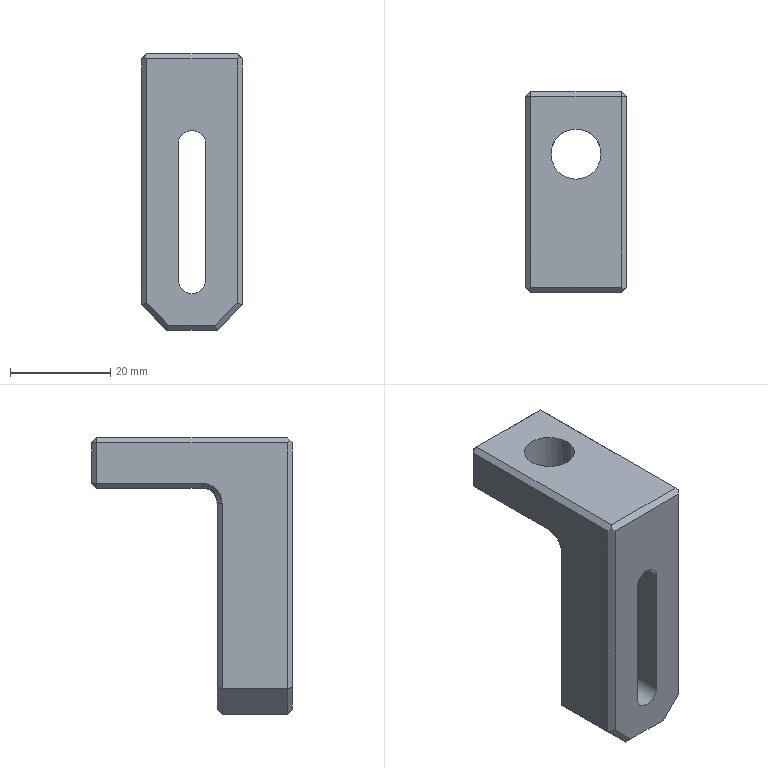Part | Creo | 1 solid | 47 faces | box 20 x 40 x 55 mm | volume 16524 mm3 | plane 38 | cylinder 7 | cone 2 | commonest cylinder face diameters 10 x4 5.5 x2 6 x1
STEP:
#1=CARTESIAN_POINT('',(-227.177,414.995,-19.5));
#2=VERTEX_POINT('',#1);
#3=CARTESIAN_POINT('',(-209.177,414.995,-19.5));
#4=VERTEX_POINT('',#3);
#5=CARTESIAN_POINT('',(-227.177,414.995,-19.5));
#6=DIRECTION('',(1.,0.,0.));
#7=VECTOR('',#6,18.);
#8=LINE('',#5,#7);
#9=EDGE_CURVE('',#2,#4,#8,.T.);
#10=ORIENTED_EDGE('',*,*,#9,.T.);
#11=CARTESIAN_POINT('',(-209.177,414.995,-11.5));
#12=VERTEX_POINT('',#11);
#13=CARTESIAN_POINT('',(-209.177,414.995,-19.5));
#14=DIRECTION('',(0.,0.,1.));
#15=VECTOR('',#14,8.);
#16=LINE('',#13,#15);
#17=EDGE_CURVE('',#4,#12,#16,.T.);
#18=ORIENTED_EDGE('',*,*,#17,.T.);
#19=CARTESIAN_POINT('',(-227.177,414.995,-11.5));
#20=VERTEX_POINT('',#19);
#21=CARTESIAN_POINT('',(-209.177,414.995,-11.5));
#22=DIRECTION('',(-1.,0.,0.));
#23=VECTOR('',#22,18.);
#24=LINE('',#21,#23);
#25=EDGE_CURVE('',#12,#20,#24,.T.);
#26=ORIENTED_EDGE('',*,*,#25,.T.);
#27=CARTESIAN_POINT('',(-227.177,414.995,-11.5));
#28=DIRECTION('',(0.,0.,-1.));
#29=VECTOR('',#28,8.);
#30=LINE('',#27,#29);
#31=EDGE_CURVE('',#20,#2,#30,.T.);
#32=ORIENTED_EDGE('',*,*,#31,.T.);
#33=EDGE_LOOP('',(#10,#18,#26,#32));
#34=FACE_OUTER_BOUND('',#33,.F.);
#35=CARTESIAN_POINT('',(-218.177,414.995,-33.));
#36=DIRECTION('',(0.,1.,0.));
#37=DIRECTION('',(0.,0.,-1.));
#38=AXIS2_PLACEMENT_3D('',#35,#36,#37);
#39=PLANE('',#38);
#40=ADVANCED_FACE('',(#34),#39,.T.);
#41=CARTESIAN_POINT('',(-209.177,413.995,-20.5));
#42=VERTEX_POINT('',#41);
#43=CARTESIAN_POINT('',(-209.177,413.995,-20.5));
#44=DIRECTION('',(0.,0.7071,0.7071));
#45=VECTOR('',#44,1.414);
#46=LINE('',#43,#45);
#47=EDGE_CURVE('',#42,#4,#46,.T.);
#48=ORIENTED_EDGE('',*,*,#47,.T.);
#49=ORIENTED_EDGE('',*,*,#9,.F.);
#50=CARTESIAN_POINT('',(-227.177,413.995,-20.5));
#51=VERTEX_POINT('',#50);
#52=CARTESIAN_POINT('',(-227.177,413.995,-20.5));
#53=DIRECTION('',(0.,0.7071,0.7071));
#54=VECTOR('',#53,1.414);
#55=LINE('',#52,#54);
#56=EDGE_CURVE('',#51,#2,#55,.T.);
#57=ORIENTED_EDGE('',*,*,#56,.F.);
#58=CARTESIAN_POINT('',(-209.177,413.995,-20.5));
#59=DIRECTION('',(-1.,0.,0.));
#60=VECTOR('',#59,18.);
#61=LINE('',#58,#60);
#62=EDGE_CURVE('',#42,#51,#61,.T.);
#63=ORIENTED_EDGE('',*,*,#62,.F.);
#64=EDGE_LOOP('',(#48,#49,#57,#63));
#65=FACE_OUTER_BOUND('',#64,.F.);
#66=CARTESIAN_POINT('',(-218.177,413.995,-20.5));
#67=DIRECTION('',(0.,0.7071,-0.7071));
#68=DIRECTION('',(1.,0.,0.));
#69=AXIS2_PLACEMENT_3D('',#66,#67,#68);
#70=PLANE('',#69);
#71=ADVANCED_FACE('',(#65),#70,.T.);
#72=CARTESIAN_POINT('',(-208.177,413.995,-19.5));
#73=VERTEX_POINT('',#72);
#74=CARTESIAN_POINT('',(-209.177,414.995,-19.5));
#75=DIRECTION('',(0.7071,-0.7071,0.));
#76=VECTOR('',#75,1.414);
#77=LINE('',#74,#76);
#78=EDGE_CURVE('',#4,#73,#77,.T.);
#79=ORIENTED_EDGE('',*,*,#78,.F.);
#80=ORIENTED_EDGE('',*,*,#47,.F.);
#81=CARTESIAN_POINT('',(-208.177,413.995,-19.5));
#82=DIRECTION('',(-0.7071,0.,-0.7071));
#83=VECTOR('',#82,1.414);
#84=LINE('',#81,#83);
#85=EDGE_CURVE('',#73,#42,#84,.T.);
#86=ORIENTED_EDGE('',*,*,#85,.F.);
#87=EDGE_LOOP('',(#79,#80,#86));
#88=FACE_OUTER_BOUND('',#87,.F.);
#89=CARTESIAN_POINT('',(-209.177,413.995,-20.5));
#90=DIRECTION('',(0.5774,0.5774,-0.5774));
#91=DIRECTION('',(0.,0.7071,0.7071));
#92=AXIS2_PLACEMENT_3D('',#89,#90,#91);
#93=PLANE('',#92);
#94=ADVANCED_FACE('',(#88),#93,.T.);
#95=CARTESIAN_POINT('',(-208.177,413.995,-11.5));
#96=VERTEX_POINT('',#95);
#97=CARTESIAN_POINT('',(-208.177,413.995,-11.5));
#98=DIRECTION('',(-0.7071,0.7071,0.));
#99=VECTOR('',#98,1.414);
#100=LINE('',#97,#99);
#101=EDGE_CURVE('',#96,#12,#100,.T.);
#102=ORIENTED_EDGE('',*,*,#101,.T.);
#103=ORIENTED_EDGE('',*,*,#17,.F.);
#104=ORIENTED_EDGE('',*,*,#78,.T.);
#105=CARTESIAN_POINT('',(-208.177,413.995,-11.5));
#106=DIRECTION('',(0.,0.,-1.));
#107=VECTOR('',#106,8.);
#108=LINE('',#105,#107);
#109=EDGE_CURVE('',#96,#73,#108,.T.);
#110=ORIENTED_EDGE('',*,*,#109,.F.);
#111=EDGE_LOOP('',(#102,#103,#104,#110));
#112=FACE_OUTER_BOUND('',#111,.F.);
#113=CARTESIAN_POINT('',(-208.177,413.995,-33.));
#114=DIRECTION('',(-0.7071,-0.7071,0.));
#115=DIRECTION('',(0.,0.,-1.));
#116=AXIS2_PLACEMENT_3D('',#113,#114,#115);
#117=PLANE('',#116);
#118=ADVANCED_FACE('',(#112),#117,.F.);
#119=CARTESIAN_POINT('',(-209.177,413.995,-10.5));
#120=VERTEX_POINT('',#119);
#121=CARTESIAN_POINT('',(-209.177,413.995,-10.5));
#122=DIRECTION('',(0.7071,0.,-0.7071));
#123=VECTOR('',#122,1.414);
#124=LINE('',#121,#123);
#125=EDGE_CURVE('',#120,#96,#124,.T.);
#126=ORIENTED_EDGE('',*,*,#125,.F.);
#127=CARTESIAN_POINT('',(-209.177,414.995,-11.5));
#128=DIRECTION('',(0.,-0.7071,0.7071));
#129=VECTOR('',#128,1.414);
#130=LINE('',#127,#129);
#131=EDGE_CURVE('',#12,#120,#130,.T.);
#132=ORIENTED_EDGE('',*,*,#131,.F.);
#133=ORIENTED_EDGE('',*,*,#101,.F.);
#134=EDGE_LOOP('',(#126,#132,#133));
#135=FACE_OUTER_BOUND('',#134,.F.);
#136=CARTESIAN_POINT('',(-208.177,413.995,-11.5));
#137=DIRECTION('',(0.5774,0.5774,0.5774));
#138=DIRECTION('',(0.,-0.7071,0.7071));
#139=AXIS2_PLACEMENT_3D('',#136,#137,#138);
#140=PLANE('',#139);
#141=ADVANCED_FACE('',(#135),#140,.T.);
#142=CARTESIAN_POINT('',(-209.177,375.995,-10.5));
#143=VERTEX_POINT('',#142);
#144=CARTESIAN_POINT('',(-209.177,413.995,-10.5));
#145=DIRECTION('',(0.,-1.,0.));
#146=VECTOR('',#145,38.);
#147=LINE('',#144,#146);
#148=EDGE_CURVE('',#120,#143,#147,.T.);
#149=ORIENTED_EDGE('',*,*,#148,.F.);
#150=ORIENTED_EDGE('',*,*,#125,.T.);
#151=CARTESIAN_POINT('',(-208.177,375.995,-11.5));
#152=VERTEX_POINT('',#151);
#153=CARTESIAN_POINT('',(-208.177,375.995,-11.5));
#154=DIRECTION('',(0.,1.,0.));
#155=VECTOR('',#154,38.);
#156=LINE('',#153,#155);
#157=EDGE_CURVE('',#152,#96,#156,.T.);
#158=ORIENTED_EDGE('',*,*,#157,.F.);
#159=CARTESIAN_POINT('',(-208.677,375.495,-11.));
#160=VERTEX_POINT('',#159);
#161=CARTESIAN_POINT('',(-208.177,375.995,-11.5));
#162=DIRECTION('',(-0.5774,-0.5774,0.5774));
#163=VECTOR('',#162,0.866);
#164=LINE('',#161,#163);
#165=EDGE_CURVE('',#152,#160,#164,.T.);
#166=ORIENTED_EDGE('',*,*,#165,.T.);
#167=CARTESIAN_POINT('',(-208.677,375.495,-11.));
#168=DIRECTION('',(-0.5774,0.5774,0.5774));
#169=VECTOR('',#168,0.866);
#170=LINE('',#167,#169);
#171=EDGE_CURVE('',#160,#143,#170,.T.);
#172=ORIENTED_EDGE('',*,*,#171,.T.);
#173=EDGE_LOOP('',(#149,#150,#158,#166,#172));
#174=FACE_OUTER_BOUND('',#173,.F.);
#175=CARTESIAN_POINT('',(-209.177,333.995,-10.5));
#176=DIRECTION('',(-0.7071,0.,-0.7071));
#177=DIRECTION('',(0.,-1.,0.));
#178=AXIS2_PLACEMENT_3D('',#175,#176,#177);
#179=PLANE('',#178);
#180=ADVANCED_FACE('',(#174),#179,.F.);
#181=CARTESIAN_POINT('',(-227.177,375.995,-10.5));
#182=VERTEX_POINT('',#181);
#183=CARTESIAN_POINT('',(-227.177,413.995,-10.5));
#184=VERTEX_POINT('',#183);
#185=CARTESIAN_POINT('',(-227.177,375.995,-10.5));
#186=DIRECTION('',(0.,1.,0.));
#187=VECTOR('',#186,38.);
#188=LINE('',#185,#187);
#189=EDGE_CURVE('',#182,#184,#188,.T.);
#190=ORIENTED_EDGE('',*,*,#189,.T.);
#191=CARTESIAN_POINT('',(-227.177,413.995,-10.5));
#192=DIRECTION('',(1.,0.,0.));
#193=VECTOR('',#192,18.);
#194=LINE('',#191,#193);
#195=EDGE_CURVE('',#184,#120,#194,.T.);
#196=ORIENTED_EDGE('',*,*,#195,.T.);
#197=ORIENTED_EDGE('',*,*,#148,.T.);
#198=CARTESIAN_POINT('',(-209.177,375.995,-10.5));
#199=DIRECTION('',(-1.,0.,0.));
#200=VECTOR('',#199,18.);
#201=LINE('',#198,#200);
#202=EDGE_CURVE('',#143,#182,#201,.T.);
#203=ORIENTED_EDGE('',*,*,#202,.T.);
#204=EDGE_LOOP('',(#190,#196,#197,#203));
#205=FACE_OUTER_BOUND('',#204,.F.);
#206=CARTESIAN_POINT('',(-218.177,397.495,-10.5));
#207=VERTEX_POINT('',#206);
#208=CARTESIAN_POINT('',(-223.177,402.495,-10.5));
#209=VERTEX_POINT('',#208);
#210=CARTESIAN_POINT('',(-218.177,402.495,-10.5));
#211=DIRECTION('',(0.,0.,-1.));
#212=DIRECTION('',(0.,-1.,0.));
#213=AXIS2_PLACEMENT_3D('',#210,#211,#212);
#214=CIRCLE('',#213,5.);
#215=EDGE_CURVE('',#207,#209,#214,.T.);
#216=ORIENTED_EDGE('',*,*,#215,.F.);
#217=CARTESIAN_POINT('',(-213.177,402.495,-10.5));
#218=VERTEX_POINT('',#217);
#219=CARTESIAN_POINT('',(-218.177,402.495,-10.5));
#220=DIRECTION('',(0.,0.,-1.));
#221=DIRECTION('',(1.,0.,0.));
#222=AXIS2_PLACEMENT_3D('',#219,#220,#221);
#223=CIRCLE('',#222,5.);
#224=EDGE_CURVE('',#218,#207,#223,.T.);
#225=ORIENTED_EDGE('',*,*,#224,.F.);
#226=CARTESIAN_POINT('',(-218.177,402.495,-10.5));
#227=DIRECTION('',(0.,0.,-1.));
#228=DIRECTION('',(-1.,0.,0.));
#229=AXIS2_PLACEMENT_3D('',#226,#227,#228);
#230=CIRCLE('',#229,5.);
#231=EDGE_CURVE('',#209,#218,#230,.T.);
#232=ORIENTED_EDGE('',*,*,#231,.F.);
#233=EDGE_LOOP('',(#216,#225,#232));
#234=FACE_BOUND('',#233,.F.);
#235=CARTESIAN_POINT('',(-218.177,333.995,-10.5));
#236=DIRECTION('',(0.,0.,1.));
#237=DIRECTION('',(0.,1.,0.));
#238=AXIS2_PLACEMENT_3D('',#235,#236,#237);
#239=PLANE('',#238);
#240=ADVANCED_FACE('',(#205,#234),#239,.T.);
#241=ORIENTED_EDGE('',*,*,#224,.T.);
#242=ORIENTED_EDGE('',*,*,#215,.T.);
#243=CARTESIAN_POINT('',(-223.177,402.495,-20.5));
#244=VERTEX_POINT('',#243);
#245=CARTESIAN_POINT('',(-223.177,402.495,-20.5));
#246=DIRECTION('',(0.,0.,1.));
#247=VECTOR('',#246,10.);
#248=LINE('',#245,#247);
#249=EDGE_CURVE('',#244,#209,#248,.T.);
#250=ORIENTED_EDGE('',*,*,#249,.F.);
#251=CARTESIAN_POINT('',(-218.177,397.495,-20.5));
#252=VERTEX_POINT('',#251);
#253=CARTESIAN_POINT('',(-218.177,402.495,-20.5));
#254=DIRECTION('',(0.,0.,1.));
#255=DIRECTION('',(-1.,0.,0.));
#256=AXIS2_PLACEMENT_3D('',#253,#254,#255);
#257=CIRCLE('',#256,5.);
#258=EDGE_CURVE('',#244,#252,#257,.T.);
#259=ORIENTED_EDGE('',*,*,#258,.T.);
#260=CARTESIAN_POINT('',(-213.177,402.495,-20.5));
#261=VERTEX_POINT('',#260);
#262=CARTESIAN_POINT('',(-218.177,402.495,-20.5));
#263=DIRECTION('',(0.,0.,1.));
#264=DIRECTION('',(0.,-1.,0.));
#265=AXIS2_PLACEMENT_3D('',#262,#263,#264);
#266=CIRCLE('',#265,5.);
#267=EDGE_CURVE('',#252,#261,#266,.T.);
#268=ORIENTED_EDGE('',*,*,#267,.T.);
#269=CARTESIAN_POINT('',(-213.177,402.495,-20.5));
#270=DIRECTION('',(0.,0.,1.));
#271=VECTOR('',#270,10.);
#272=LINE('',#269,#271);
#273=EDGE_CURVE('',#261,#218,#272,.T.);
#274=ORIENTED_EDGE('',*,*,#273,.T.);
#275=EDGE_LOOP('',(#241,#242,#250,#259,#268,#274));
#276=FACE_OUTER_BOUND('',#275,.F.);
#277=CARTESIAN_POINT('',(-218.177,402.495,-25.5));
#278=DIRECTION('',(0.,0.,1.));
#279=DIRECTION('',(-1.,0.,0.));
#280=AXIS2_PLACEMENT_3D('',#277,#278,#279);
#281=CYLINDRICAL_SURFACE('',#280,5.);
#282=ADVANCED_FACE('',(#276),#281,.F.);
#283=ORIENTED_EDGE('',*,*,#231,.T.);
#284=ORIENTED_EDGE('',*,*,#273,.F.);
#285=CARTESIAN_POINT('',(-218.177,407.495,-20.5));
#286=VERTEX_POINT('',#285);
#287=CARTESIAN_POINT('',(-218.177,402.495,-20.5));
#288=DIRECTION('',(0.,0.,1.));
#289=DIRECTION('',(1.,0.,0.));
#290=AXIS2_PLACEMENT_3D('',#287,#288,#289);
#291=CIRCLE('',#290,5.);
#292=EDGE_CURVE('',#261,#286,#291,.T.);
#293=ORIENTED_EDGE('',*,*,#292,.T.);
#294=CARTESIAN_POINT('',(-218.177,402.495,-20.5));
#295=DIRECTION('',(0.,0.,1.));
#296=DIRECTION('',(0.,1.,0.));
#297=AXIS2_PLACEMENT_3D('',#294,#295,#296);
#298=CIRCLE('',#297,5.);
#299=EDGE_CURVE('',#286,#244,#298,.T.);
#300=ORIENTED_EDGE('',*,*,#299,.T.);
#301=ORIENTED_EDGE('',*,*,#249,.T.);
#302=EDGE_LOOP('',(#283,#284,#293,#300,#301));
#303=FACE_OUTER_BOUND('',#302,.F.);
#304=CARTESIAN_POINT('',(-218.177,402.495,-25.5));
#305=DIRECTION('',(0.,0.,1.));
#306=DIRECTION('',(-1.,0.,0.));
#307=AXIS2_PLACEMENT_3D('',#304,#305,#306);
#308=CYLINDRICAL_SURFACE('',#307,5.);
#309=ADVANCED_FACE('',(#303),#308,.F.);
#310=CARTESIAN_POINT('',(-227.177,392.995,-20.5));
#311=VERTEX_POINT('',#310);
#312=CARTESIAN_POINT('',(-209.177,392.995,-20.5));
#313=VERTEX_POINT('',#312);
#314=CARTESIAN_POINT('',(-227.177,392.995,-20.5));
#315=DIRECTION('',(1.,0.,0.));
#316=VECTOR('',#315,18.);
#317=LINE('',#314,#316);
#318=EDGE_CURVE('',#311,#313,#317,.T.);
#319=ORIENTED_EDGE('',*,*,#318,.T.);
#320=CARTESIAN_POINT('',(-209.177,392.995,-20.5));
#321=DIRECTION('',(0.,1.,0.));
#322=VECTOR('',#321,21.);
#323=LINE('',#320,#322);
#324=EDGE_CURVE('',#313,#42,#323,.T.);
#325=ORIENTED_EDGE('',*,*,#324,.T.);
#326=ORIENTED_EDGE('',*,*,#62,.T.);
#327=CARTESIAN_POINT('',(-227.177,413.995,-20.5));
#328=DIRECTION('',(0.,-1.,0.));
#329=VECTOR('',#328,21.);
#330=LINE('',#327,#329);
#331=EDGE_CURVE('',#51,#311,#330,.T.);
#332=ORIENTED_EDGE('',*,*,#331,.T.);
#333=EDGE_LOOP('',(#319,#325,#326,#332));
#334=FACE_OUTER_BOUND('',#333,.F.);
#335=ORIENTED_EDGE('',*,*,#299,.F.);
#336=ORIENTED_EDGE('',*,*,#292,.F.);
#337=ORIENTED_EDGE('',*,*,#267,.F.);
#338=ORIENTED_EDGE('',*,*,#258,.F.);
#339=EDGE_LOOP('',(#335,#336,#337,#338));
#340=FACE_BOUND('',#339,.F.);
#341=CARTESIAN_POINT('',(-218.177,389.995,-20.5));
#342=DIRECTION('',(0.,0.,1.));
#343=DIRECTION('',(0.,1.,0.));
#344=AXIS2_PLACEMENT_3D('',#341,#342,#343);
#345=PLANE('',#344);
#346=ADVANCED_FACE('',(#334,#340),#345,.F.);
#347=CARTESIAN_POINT('',(-218.177,389.995,-23.5));
#348=VERTEX_POINT('',#347);
#349=CARTESIAN_POINT('',(-227.177,389.995,-23.5));
#350=VERTEX_POINT('',#349);
#351=CARTESIAN_POINT('',(-218.177,389.995,-23.5));
#352=DIRECTION('',(-1.,0.,0.));
#353=VECTOR('',#352,9.);
#354=LINE('',#351,#353);
#355=EDGE_CURVE('',#348,#350,#354,.T.);
#356=ORIENTED_EDGE('',*,*,#355,.F.);
#357=CARTESIAN_POINT('',(-209.177,389.995,-23.5));
#358=VERTEX_POINT('',#357);
#359=CARTESIAN_POINT('',(-209.177,389.995,-23.5));
#360=DIRECTION('',(-1.,0.,0.));
#361=VECTOR('',#360,9.);
#362=LINE('',#359,#361);
#363=EDGE_CURVE('',#358,#348,#362,.T.);
#364=ORIENTED_EDGE('',*,*,#363,.F.);
#365=CARTESIAN_POINT('',(-209.177,392.995,-23.5));
#366=DIRECTION('',(-1.,0.,0.));
#367=DIRECTION('',(0.,-1.,0.));
#368=AXIS2_PLACEMENT_3D('',#365,#366,#367);
#369=CIRCLE('',#368,3.);
#370=EDGE_CURVE('',#358,#313,#369,.T.);
#371=ORIENTED_EDGE('',*,*,#370,.T.);
#372=ORIENTED_EDGE('',*,*,#318,.F.);
#373=CARTESIAN_POINT('',(-227.177,392.995,-23.5));
#374=DIRECTION('',(1.,0.,0.));
#375=DIRECTION('',(0.,0.,1.));
#376=AXIS2_PLACEMENT_3D('',#373,#374,#375);
#377=CIRCLE('',#376,3.);
#378=EDGE_CURVE('',#311,#350,#377,.T.);
#379=ORIENTED_EDGE('',*,*,#378,.T.);
#380=EDGE_LOOP('',(#356,#364,#371,#372,#379));
#381=FACE_OUTER_BOUND('',#380,.F.);
#382=CARTESIAN_POINT('',(-218.177,392.995,-23.5));
#383=DIRECTION('',(1.,0.,0.));
#384=DIRECTION('',(0.,1.,0.));
#385=AXIS2_PLACEMENT_3D('',#382,#383,#384);
#386=CYLINDRICAL_SURFACE('',#385,3.);
#387=ADVANCED_FACE('',(#381),#386,.F.);
#388=CARTESIAN_POINT('',(-222.763,389.995,-64.5));
#389=VERTEX_POINT('',#388);
#390=CARTESIAN_POINT('',(-227.177,389.995,-60.086));
#391=VERTEX_POINT('',#390);
#392=CARTESIAN_POINT('',(-222.763,389.995,-64.5));
#393=DIRECTION('',(-0.7071,0.,0.7071));
#394=VECTOR('',#393,6.243);
#395=LINE('',#392,#394);
#396=EDGE_CURVE('',#389,#391,#395,.T.);
#397=ORIENTED_EDGE('',*,*,#396,.F.);
#398=CARTESIAN_POINT('',(-213.591,389.995,-64.5));
#399=VERTEX_POINT('',#398);
#400=CARTESIAN_POINT('',(-222.763,389.995,-64.5));
#401=DIRECTION('',(1.,0.,0.));
#402=VECTOR('',#401,9.172);
#403=LINE('',#400,#402);
#404=EDGE_CURVE('',#389,#399,#403,.T.);
#405=ORIENTED_EDGE('',*,*,#404,.T.);
#406=CARTESIAN_POINT('',(-209.177,389.995,-60.086));
#407=VERTEX_POINT('',#406);
#408=CARTESIAN_POINT('',(-209.177,389.995,-60.086));
#409=DIRECTION('',(-0.7071,0.,-0.7071));
#410=VECTOR('',#409,6.243);
#411=LINE('',#408,#410);
#412=EDGE_CURVE('',#407,#399,#411,.T.);
#413=ORIENTED_EDGE('',*,*,#412,.F.);
#414=CARTESIAN_POINT('',(-209.177,389.995,-60.086));
#415=DIRECTION('',(0.,0.,1.));
#416=VECTOR('',#415,36.586);
#417=LINE('',#414,#416);
#418=EDGE_CURVE('',#407,#358,#417,.T.);
#419=ORIENTED_EDGE('',*,*,#418,.T.);
#420=ORIENTED_EDGE('',*,*,#363,.T.);
#421=CARTESIAN_POINT('',(-213.177,389.995,-28.5));
#422=VERTEX_POINT('',#421);
#423=CARTESIAN_POINT('',(-218.177,389.995,-28.5));
#424=DIRECTION('',(0.,-1.,0.));
#425=DIRECTION('',(1.,0.,0.));
#426=AXIS2_PLACEMENT_3D('',#423,#424,#425);
#427=CIRCLE('',#426,5.);
#428=EDGE_CURVE('',#422,#348,#427,.T.);
#429=ORIENTED_EDGE('',*,*,#428,.F.);
#430=CARTESIAN_POINT('',(-213.177,389.995,-55.5));
#431=VERTEX_POINT('',#430);
#432=CARTESIAN_POINT('',(-213.177,389.995,-28.5));
#433=DIRECTION('',(0.,0.,-1.));
#434=VECTOR('',#433,27.);
#435=LINE('',#432,#434);
#436=EDGE_CURVE('',#422,#431,#435,.T.);
#437=ORIENTED_EDGE('',*,*,#436,.T.);
#438=CARTESIAN_POINT('',(-218.177,389.995,-60.5));
#439=VERTEX_POINT('',#438);
#440=CARTESIAN_POINT('',(-218.177,389.995,-55.5));
#441=DIRECTION('',(0.,-1.,0.));
#442=DIRECTION('',(0.,0.,-1.));
#443=AXIS2_PLACEMENT_3D('',#440,#441,#442);
#444=CIRCLE('',#443,5.);
#445=EDGE_CURVE('',#439,#431,#444,.T.);
#446=ORIENTED_EDGE('',*,*,#445,.F.);
#447=CARTESIAN_POINT('',(-223.177,389.995,-55.5));
#448=VERTEX_POINT('',#447);
#449=CARTESIAN_POINT('',(-218.177,389.995,-55.5));
#450=DIRECTION('',(0.,-1.,0.));
#451=DIRECTION('',(-1.,0.,0.));
#452=AXIS2_PLACEMENT_3D('',#449,#450,#451);
#453=CIRCLE('',#452,5.);
#454=EDGE_CURVE('',#448,#439,#453,.T.);
#455=ORIENTED_EDGE('',*,*,#454,.F.);
#456=CARTESIAN_POINT('',(-223.177,389.995,-28.5));
#457=VERTEX_POINT('',#456);
#458=CARTESIAN_POINT('',(-223.177,389.995,-55.5));
#459=DIRECTION('',(0.,0.,1.));
#460=VECTOR('',#459,27.);
#461=LINE('',#458,#460);
#462=EDGE_CURVE('',#448,#457,#461,.T.);
#463=ORIENTED_EDGE('',*,*,#462,.T.);
#464=CARTESIAN_POINT('',(-218.177,389.995,-28.5));
#465=DIRECTION('',(0.,-1.,0.));
#466=DIRECTION('',(0.,0.,1.));
#467=AXIS2_PLACEMENT_3D('',#464,#465,#466);
#468=CIRCLE('',#467,5.);
#469=EDGE_CURVE('',#348,#457,#468,.T.);
#470=ORIENTED_EDGE('',*,*,#469,.F.);
#471=ORIENTED_EDGE('',*,*,#355,.T.);
#472=CARTESIAN_POINT('',(-227.177,389.995,-23.5));
#473=DIRECTION('',(0.,0.,-1.));
#474=VECTOR('',#473,36.586);
#475=LINE('',#472,#474);
#476=EDGE_CURVE('',#350,#391,#475,.T.);
#477=ORIENTED_EDGE('',*,*,#476,.T.);
#478=EDGE_LOOP('',(#397,#405,#413,#419,#420,#429,#437,#446,#455,#463,#470,#471,#477));
#479=FACE_OUTER_BOUND('',#478,.F.);
#480=CARTESIAN_POINT('',(-218.177,389.995,-48.));
#481=DIRECTION('',(0.,-1.,0.));
#482=DIRECTION('',(0.,0.,1.));
#483=AXIS2_PLACEMENT_3D('',#480,#481,#482);
#484=PLANE('',#483);
#485=ADVANCED_FACE('',(#479),#484,.F.);
#486=CARTESIAN_POINT('',(-223.177,388.995,-65.5));
#487=VERTEX_POINT('',#486);
#488=CARTESIAN_POINT('',(-223.177,388.995,-65.5));
#489=DIRECTION('',(0.2811,0.6786,0.6786));
#490=VECTOR('',#489,1.474);
#491=LINE('',#488,#490);
#492=EDGE_CURVE('',#487,#389,#491,.T.);
#493=ORIENTED_EDGE('',*,*,#492,.T.);
#494=ORIENTED_EDGE('',*,*,#396,.T.);
#495=CARTESIAN_POINT('',(-228.177,388.995,-60.5));
#496=VERTEX_POINT('',#495);
#497=CARTESIAN_POINT('',(-228.177,388.995,-60.5));
#498=DIRECTION('',(0.6786,0.6786,0.2811));
#499=VECTOR('',#498,1.474);
#500=LINE('',#497,#499);
#501=EDGE_CURVE('',#496,#391,#500,.T.);
#502=ORIENTED_EDGE('',*,*,#501,.F.);
#503=CARTESIAN_POINT('',(-223.177,388.995,-65.5));
#504=DIRECTION('',(-0.7071,0.,0.7071));
#505=VECTOR('',#504,7.071);
#506=LINE('',#503,#505);
#507=EDGE_CURVE('',#487,#496,#506,.T.);
#508=ORIENTED_EDGE('',*,*,#507,.F.);
#509=EDGE_LOOP('',(#493,#494,#502,#508));
#510=FACE_OUTER_BOUND('',#509,.F.);
#511=CARTESIAN_POINT('',(-228.72,389.995,-58.543));
#512=DIRECTION('',(0.5,-0.7071,0.5));
#513=DIRECTION('',(0.7071,0.,-0.7071));
#514=AXIS2_PLACEMENT_3D('',#511,#512,#513);
#515=PLANE('',#514);
#516=ADVANCED_FACE('',(#510),#515,.F.);
#517=CARTESIAN_POINT('',(-213.177,388.995,-65.5));
#518=VERTEX_POINT('',#517);
#519=CARTESIAN_POINT('',(-213.177,388.995,-65.5));
#520=DIRECTION('',(-0.2811,0.6786,0.6786));
#521=VECTOR('',#520,1.474);
#522=LINE('',#519,#521);
#523=EDGE_CURVE('',#518,#399,#522,.T.);
#524=ORIENTED_EDGE('',*,*,#523,.T.);
#525=ORIENTED_EDGE('',*,*,#404,.F.);
#526=ORIENTED_EDGE('',*,*,#492,.F.);
#527=CARTESIAN_POINT('',(-213.177,388.995,-65.5));
#528=DIRECTION('',(-1.,0.,0.));
#529=VECTOR('',#528,10.);
#530=LINE('',#527,#529);
#531=EDGE_CURVE('',#518,#487,#530,.T.);
#532=ORIENTED_EDGE('',*,*,#531,.F.);
#533=EDGE_LOOP('',(#524,#525,#526,#532));
#534=FACE_OUTER_BOUND('',#533,.F.);
#535=CARTESIAN_POINT('',(-218.177,389.995,-64.5));
#536=DIRECTION('',(0.,0.7071,-0.7071));
#537=DIRECTION('',(-1.,0.,0.));
#538=AXIS2_PLACEMENT_3D('',#535,#536,#537);
#539=PLANE('',#538);
#540=ADVANCED_FACE('',(#534),#539,.T.);
#541=CARTESIAN_POINT('',(-208.177,388.995,-60.5));
#542=VERTEX_POINT('',#541);
#543=CARTESIAN_POINT('',(-209.177,389.995,-60.086));
#544=DIRECTION('',(0.6786,-0.6786,-0.2811));
#545=VECTOR('',#544,1.474);
#546=LINE('',#543,#545);
#547=EDGE_CURVE('',#407,#542,#546,.T.);
#548=ORIENTED_EDGE('',*,*,#547,.F.);
#549=ORIENTED_EDGE('',*,*,#412,.T.);
#550=ORIENTED_EDGE('',*,*,#523,.F.);
#551=CARTESIAN_POINT('',(-208.177,388.995,-60.5));
#552=DIRECTION('',(-0.7071,0.,-0.7071));
#553=VECTOR('',#552,7.071);
#554=LINE('',#551,#553);
#555=EDGE_CURVE('',#542,#518,#554,.T.);
#556=ORIENTED_EDGE('',*,*,#555,.F.);
#557=EDGE_LOOP('',(#548,#549,#550,#556));
#558=FACE_OUTER_BOUND('',#557,.F.);
#559=CARTESIAN_POINT('',(-207.634,389.995,-58.543));
#560=DIRECTION('',(-0.5,-0.7071,0.5));
#561=DIRECTION('',(0.7071,0.,0.7071));
#562=AXIS2_PLACEMENT_3D('',#559,#560,#561);
#563=PLANE('',#562);
#564=ADVANCED_FACE('',(#558),#563,.F.);
#565=ORIENTED_EDGE('',*,*,#547,.T.);
#566=CARTESIAN_POINT('',(-208.177,388.995,-23.5));
#567=VERTEX_POINT('',#566);
#568=CARTESIAN_POINT('',(-208.177,388.995,-23.5));
#569=DIRECTION('',(0.,0.,-1.));
#570=VECTOR('',#569,37.);
#571=LINE('',#568,#570);
#572=EDGE_CURVE('',#567,#542,#571,.T.);
#573=ORIENTED_EDGE('',*,*,#572,.F.);
#574=CARTESIAN_POINT('',(-208.177,388.995,-23.5));
#575=DIRECTION('',(-0.7071,0.7071,0.));
#576=VECTOR('',#575,1.414);
#577=LINE('',#574,#576);
#578=EDGE_CURVE('',#567,#358,#577,.T.);
#579=ORIENTED_EDGE('',*,*,#578,.T.);
#580=ORIENTED_EDGE('',*,*,#418,.F.);
#581=EDGE_LOOP('',(#565,#573,#579,#580));
#582=FACE_OUTER_BOUND('',#581,.F.);
#583=CARTESIAN_POINT('',(-209.177,389.995,-48.));
#584=DIRECTION('',(0.7071,0.7071,0.));
#585=DIRECTION('',(0.,0.,-1.));
#586=AXIS2_PLACEMENT_3D('',#583,#584,#585);
#587=PLANE('',#586);
#588=ADVANCED_FACE('',(#582),#587,.T.);
#589=CARTESIAN_POINT('',(-208.177,375.995,-60.5));
#590=VERTEX_POINT('',#589);
#591=CARTESIAN_POINT('',(-208.177,388.995,-60.5));
#592=DIRECTION('',(0.,-1.,0.));
#593=VECTOR('',#592,13.);
#594=LINE('',#591,#593);
#595=EDGE_CURVE('',#542,#590,#594,.T.);
#596=ORIENTED_EDGE('',*,*,#595,.T.);
#597=CARTESIAN_POINT('',(-208.177,375.995,-60.5));
#598=DIRECTION('',(0.,0.,1.));
#599=VECTOR('',#598,49.);
#600=LINE('',#597,#599);
#601=EDGE_CURVE('',#590,#152,#600,.T.);
#602=ORIENTED_EDGE('',*,*,#601,.T.);
#603=ORIENTED_EDGE('',*,*,#157,.T.);
#604=ORIENTED_EDGE('',*,*,#109,.T.);
#605=CARTESIAN_POINT('',(-208.177,392.995,-19.5));
#606=VERTEX_POINT('',#605);
#607=CARTESIAN_POINT('',(-208.177,413.995,-19.5));
#608=DIRECTION('',(0.,-1.,0.));
#609=VECTOR('',#608,21.);
#610=LINE('',#607,#609);
#611=EDGE_CURVE('',#73,#606,#610,.T.);
#612=ORIENTED_EDGE('',*,*,#611,.T.);
#613=CARTESIAN_POINT('',(-208.177,392.995,-23.5));
#614=DIRECTION('',(-1.,0.,0.));
#615=DIRECTION('',(0.,-1.,0.));
#616=AXIS2_PLACEMENT_3D('',#613,#614,#615);
#617=CIRCLE('',#616,4.);
#618=EDGE_CURVE('',#567,#606,#617,.T.);
#619=ORIENTED_EDGE('',*,*,#618,.F.);
#620=ORIENTED_EDGE('',*,*,#572,.T.);
#621=EDGE_LOOP('',(#596,#602,#603,#604,#612,#619,#620));
#622=FACE_OUTER_BOUND('',#621,.F.);
#623=CARTESIAN_POINT('',(-208.177,333.995,-33.));
#624=DIRECTION('',(1.,0.,0.));
#625=DIRECTION('',(0.,-1.,0.));
#626=AXIS2_PLACEMENT_3D('',#623,#624,#625);
#627=PLANE('',#626);
#628=ADVANCED_FACE('',(#622),#627,.T.);
#629=CARTESIAN_POINT('',(-213.177,375.995,-65.5));
#630=VERTEX_POINT('',#629);
#631=CARTESIAN_POINT('',(-213.177,375.995,-65.5));
#632=DIRECTION('',(0.,1.,0.));
#633=VECTOR('',#632,13.);
#634=LINE('',#631,#633);
#635=EDGE_CURVE('',#630,#518,#634,.T.);
#636=ORIENTED_EDGE('',*,*,#635,.F.);
#637=CARTESIAN_POINT('',(-213.177,375.995,-65.5));
#638=DIRECTION('',(0.7071,0.,0.7071));
#639=VECTOR('',#638,7.071);
#640=LINE('',#637,#639);
#641=EDGE_CURVE('',#630,#590,#640,.T.);
#642=ORIENTED_EDGE('',*,*,#641,.T.);
#643=ORIENTED_EDGE('',*,*,#595,.F.);
#644=ORIENTED_EDGE('',*,*,#555,.T.);
#645=EDGE_LOOP('',(#636,#642,#643,#644));
#646=FACE_OUTER_BOUND('',#645,.F.);
#647=CARTESIAN_POINT('',(-208.177,333.995,-60.5));
#648=DIRECTION('',(-0.7071,0.,0.7071));
#649=DIRECTION('',(0.,-1.,0.));
#650=AXIS2_PLACEMENT_3D('',#647,#648,#649);
#651=PLANE('',#650);
#652=ADVANCED_FACE('',(#646),#651,.F.);
#653=CARTESIAN_POINT('',(-223.177,375.995,-65.5));
#654=VERTEX_POINT('',#653);
#655=CARTESIAN_POINT('',(-223.177,388.995,-65.5));
#656=DIRECTION('',(0.,-1.,0.));
#657=VECTOR('',#656,13.);
#658=LINE('',#655,#657);
#659=EDGE_CURVE('',#487,#654,#658,.T.);
#660=ORIENTED_EDGE('',*,*,#659,.T.);
#661=CARTESIAN_POINT('',(-223.177,375.995,-65.5));
#662=DIRECTION('',(1.,0.,0.));
#663=VECTOR('',#662,10.);
#664=LINE('',#661,#663);
#665=EDGE_CURVE('',#654,#630,#664,.T.);
#666=ORIENTED_EDGE('',*,*,#665,.T.);
#667=ORIENTED_EDGE('',*,*,#635,.T.);
#668=ORIENTED_EDGE('',*,*,#531,.T.);
#669=EDGE_LOOP('',(#660,#666,#667,#668));
#670=FACE_OUTER_BOUND('',#669,.F.);
#671=CARTESIAN_POINT('',(-218.177,333.995,-65.5));
#672=DIRECTION('',(0.,0.,-1.));
#673=DIRECTION('',(0.,-1.,0.));
#674=AXIS2_PLACEMENT_3D('',#671,#672,#673);
#675=PLANE('',#674);
#676=ADVANCED_FACE('',(#670),#675,.T.);
#677=ORIENTED_EDGE('',*,*,#659,.F.);
#678=ORIENTED_EDGE('',*,*,#507,.T.);
#679=CARTESIAN_POINT('',(-228.177,375.995,-60.5));
#680=VERTEX_POINT('',#679);
#681=CARTESIAN_POINT('',(-228.177,375.995,-60.5));
#682=DIRECTION('',(0.,1.,0.));
#683=VECTOR('',#682,13.);
#684=LINE('',#681,#683);
#685=EDGE_CURVE('',#680,#496,#684,.T.);
#686=ORIENTED_EDGE('',*,*,#685,.F.);
#687=CARTESIAN_POINT('',(-228.177,375.995,-60.5));
#688=DIRECTION('',(0.7071,0.,-0.7071));
#689=VECTOR('',#688,7.071);
#690=LINE('',#687,#689);
#691=EDGE_CURVE('',#680,#654,#690,.T.);
#692=ORIENTED_EDGE('',*,*,#691,.T.);
#693=EDGE_LOOP('',(#677,#678,#686,#692));
#694=FACE_OUTER_BOUND('',#693,.F.);
#695=CARTESIAN_POINT('',(-223.177,333.995,-65.5));
#696=DIRECTION('',(0.7071,0.,0.7071));
#697=DIRECTION('',(0.,-1.,0.));
#698=AXIS2_PLACEMENT_3D('',#695,#696,#697);
#699=PLANE('',#698);
#700=ADVANCED_FACE('',(#694),#699,.F.);
#701=CARTESIAN_POINT('',(-228.177,392.995,-19.5));
#702=VERTEX_POINT('',#701);
#703=CARTESIAN_POINT('',(-228.177,388.995,-23.5));
#704=VERTEX_POINT('',#703);
#705=CARTESIAN_POINT('',(-228.177,392.995,-23.5));
#706=DIRECTION('',(1.,0.,0.));
#707=DIRECTION('',(0.,0.,1.));
#708=AXIS2_PLACEMENT_3D('',#705,#706,#707);
#709=CIRCLE('',#708,4.);
#710=EDGE_CURVE('',#702,#704,#709,.T.);
#711=ORIENTED_EDGE('',*,*,#710,.F.);
#712=CARTESIAN_POINT('',(-228.177,413.995,-19.5));
#713=VERTEX_POINT('',#712);
#714=CARTESIAN_POINT('',(-228.177,392.995,-19.5));
#715=DIRECTION('',(0.,1.,0.));
#716=VECTOR('',#715,21.);
#717=LINE('',#714,#716);
#718=EDGE_CURVE('',#702,#713,#717,.T.);
#719=ORIENTED_EDGE('',*,*,#718,.T.);
#720=CARTESIAN_POINT('',(-228.177,413.995,-11.5));
#721=VERTEX_POINT('',#720);
#722=CARTESIAN_POINT('',(-228.177,413.995,-19.5));
#723=DIRECTION('',(0.,0.,1.));
#724=VECTOR('',#723,8.);
#725=LINE('',#722,#724);
#726=EDGE_CURVE('',#713,#721,#725,.T.);
#727=ORIENTED_EDGE('',*,*,#726,.T.);
#728=CARTESIAN_POINT('',(-228.177,375.995,-11.5));
#729=VERTEX_POINT('',#728);
#730=CARTESIAN_POINT('',(-228.177,413.995,-11.5));
#731=DIRECTION('',(0.,-1.,0.));
#732=VECTOR('',#731,38.);
#733=LINE('',#730,#732);
#734=EDGE_CURVE('',#721,#729,#733,.T.);
#735=ORIENTED_EDGE('',*,*,#734,.T.);
#736=CARTESIAN_POINT('',(-228.177,375.995,-11.5));
#737=DIRECTION('',(0.,0.,-1.));
#738=VECTOR('',#737,49.);
#739=LINE('',#736,#738);
#740=EDGE_CURVE('',#729,#680,#739,.T.);
#741=ORIENTED_EDGE('',*,*,#740,.T.);
#742=ORIENTED_EDGE('',*,*,#685,.T.);
#743=CARTESIAN_POINT('',(-228.177,388.995,-60.5));
#744=DIRECTION('',(0.,0.,1.));
#745=VECTOR('',#744,37.);
#746=LINE('',#743,#745);
#747=EDGE_CURVE('',#496,#704,#746,.T.);
#748=ORIENTED_EDGE('',*,*,#747,.T.);
#749=EDGE_LOOP('',(#711,#719,#727,#735,#741,#742,#748));
#750=FACE_OUTER_BOUND('',#749,.F.);
#751=CARTESIAN_POINT('',(-228.177,333.995,-33.));
#752=DIRECTION('',(-1.,0.,0.));
#753=DIRECTION('',(0.,1.,0.));
#754=AXIS2_PLACEMENT_3D('',#751,#752,#753);
#755=PLANE('',#754);
#756=ADVANCED_FACE('',(#750),#755,.T.);
#757=CARTESIAN_POINT('',(-227.177,389.995,-23.5));
#758=DIRECTION('',(-0.7071,-0.7071,0.));
#759=VECTOR('',#758,1.414);
#760=LINE('',#757,#759);
#761=EDGE_CURVE('',#350,#704,#760,.T.);
#762=ORIENTED_EDGE('',*,*,#761,.F.);
#763=ORIENTED_EDGE('',*,*,#378,.F.);
#764=CARTESIAN_POINT('',(-228.177,392.995,-19.5));
#765=DIRECTION('',(0.7071,0.,-0.7071));
#766=VECTOR('',#765,1.414);
#767=LINE('',#764,#766);
#768=EDGE_CURVE('',#702,#311,#767,.T.);
#769=ORIENTED_EDGE('',*,*,#768,.F.);
#770=ORIENTED_EDGE('',*,*,#710,.T.);
#771=EDGE_LOOP('',(#762,#763,#769,#770));
#772=FACE_OUTER_BOUND('',#771,.F.);
#773=CARTESIAN_POINT('',(-227.677,392.995,-23.5));
#774=DIRECTION('',(-1.,0.,0.));
#775=DIRECTION('',(0.,-1.,0.));
#776=AXIS2_PLACEMENT_3D('',#773,#774,#775);
#777=CONICAL_SURFACE('',#776,3.5,45.);
#778=ADVANCED_FACE('',(#772),#777,.F.);
#779=ORIENTED_EDGE('',*,*,#501,.T.);
#780=ORIENTED_EDGE('',*,*,#476,.F.);
#781=ORIENTED_EDGE('',*,*,#761,.T.);
#782=ORIENTED_EDGE('',*,*,#747,.F.);
#783=EDGE_LOOP('',(#779,#780,#781,#782));
#784=FACE_OUTER_BOUND('',#783,.F.);
#785=CARTESIAN_POINT('',(-227.177,389.995,-48.));
#786=DIRECTION('',(-0.7071,0.7071,0.));
#787=DIRECTION('',(0.,0.,1.));
#788=AXIS2_PLACEMENT_3D('',#785,#786,#787);
#789=PLANE('',#788);
#790=ADVANCED_FACE('',(#784),#789,.T.);
#791=ORIENTED_EDGE('',*,*,#768,.T.);
#792=ORIENTED_EDGE('',*,*,#331,.F.);
#793=CARTESIAN_POINT('',(-227.177,413.995,-20.5));
#794=DIRECTION('',(-0.7071,0.,0.7071));
#795=VECTOR('',#794,1.414);
#796=LINE('',#793,#795);
#797=EDGE_CURVE('',#51,#713,#796,.T.);
#798=ORIENTED_EDGE('',*,*,#797,.T.);
#799=ORIENTED_EDGE('',*,*,#718,.F.);
#800=EDGE_LOOP('',(#791,#792,#798,#799));
#801=FACE_OUTER_BOUND('',#800,.F.);
#802=CARTESIAN_POINT('',(-227.177,389.995,-20.5));
#803=DIRECTION('',(-0.7071,0.,-0.7071));
#804=DIRECTION('',(0.,1.,0.));
#805=AXIS2_PLACEMENT_3D('',#802,#803,#804);
#806=PLANE('',#805);
#807=ADVANCED_FACE('',(#801),#806,.T.);
#808=ORIENTED_EDGE('',*,*,#56,.T.);
#809=CARTESIAN_POINT('',(-228.177,413.995,-19.5));
#810=DIRECTION('',(0.7071,0.7071,0.));
#811=VECTOR('',#810,1.414);
#812=LINE('',#809,#811);
#813=EDGE_CURVE('',#713,#2,#812,.T.);
#814=ORIENTED_EDGE('',*,*,#813,.F.);
#815=ORIENTED_EDGE('',*,*,#797,.F.);
#816=EDGE_LOOP('',(#808,#814,#815));
#817=FACE_OUTER_BOUND('',#816,.F.);
#818=CARTESIAN_POINT('',(-228.177,413.995,-19.5));
#819=DIRECTION('',(-0.5774,0.5774,-0.5774));
#820=DIRECTION('',(0.,0.7071,0.7071));
#821=AXIS2_PLACEMENT_3D('',#818,#819,#820);
#822=PLANE('',#821);
#823=ADVANCED_FACE('',(#817),#822,.T.);
#824=CARTESIAN_POINT('',(-227.177,414.995,-11.5));
#825=DIRECTION('',(-0.7071,-0.7071,0.));
#826=VECTOR('',#825,1.414);
#827=LINE('',#824,#826);
#828=EDGE_CURVE('',#20,#721,#827,.T.);
#829=ORIENTED_EDGE('',*,*,#828,.T.);
#830=ORIENTED_EDGE('',*,*,#726,.F.);
#831=ORIENTED_EDGE('',*,*,#813,.T.);
#832=ORIENTED_EDGE('',*,*,#31,.F.);
#833=EDGE_LOOP('',(#829,#830,#831,#832));
#834=FACE_OUTER_BOUND('',#833,.F.);
#835=CARTESIAN_POINT('',(-228.177,413.995,-33.));
#836=DIRECTION('',(0.7071,-0.7071,0.));
#837=DIRECTION('',(0.,0.,1.));
#838=AXIS2_PLACEMENT_3D('',#835,#836,#837);
#839=PLANE('',#838);
#840=ADVANCED_FACE('',(#834),#839,.F.);
#841=CARTESIAN_POINT('',(-228.177,413.995,-11.5));
#842=DIRECTION('',(0.7071,0.,0.7071));
#843=VECTOR('',#842,1.414);
#844=LINE('',#841,#843);
#845=EDGE_CURVE('',#721,#184,#844,.T.);
#846=ORIENTED_EDGE('',*,*,#845,.F.);
#847=ORIENTED_EDGE('',*,*,#828,.F.);
#848=CARTESIAN_POINT('',(-227.177,414.995,-11.5));
#849=DIRECTION('',(0.,-0.7071,0.7071));
#850=VECTOR('',#849,1.414);
#851=LINE('',#848,#850);
#852=EDGE_CURVE('',#20,#184,#851,.T.);
#853=ORIENTED_EDGE('',*,*,#852,.T.);
#854=EDGE_LOOP('',(#846,#847,#853));
#855=FACE_OUTER_BOUND('',#854,.F.);
#856=CARTESIAN_POINT('',(-227.177,414.995,-11.5));
#857=DIRECTION('',(-0.5774,0.5774,0.5774));
#858=DIRECTION('',(0.,-0.7071,0.7071));
#859=AXIS2_PLACEMENT_3D('',#856,#857,#858);
#860=PLANE('',#859);
#861=ADVANCED_FACE('',(#855),#860,.T.);
#862=CARTESIAN_POINT('',(-227.677,375.495,-11.));
#863=VERTEX_POINT('',#862);
#864=CARTESIAN_POINT('',(-227.677,375.495,-11.));
#865=DIRECTION('',(-0.5774,0.5774,-0.5774));
#866=VECTOR('',#865,0.866);
#867=LINE('',#864,#866);
#868=EDGE_CURVE('',#863,#729,#867,.T.);
#869=ORIENTED_EDGE('',*,*,#868,.T.);
#870=ORIENTED_EDGE('',*,*,#734,.F.);
#871=ORIENTED_EDGE('',*,*,#845,.T.);
#872=ORIENTED_EDGE('',*,*,#189,.F.);
#873=CARTESIAN_POINT('',(-227.177,375.995,-10.5));
#874=DIRECTION('',(-0.5774,-0.5774,-0.5774));
#875=VECTOR('',#874,0.866);
#876=LINE('',#873,#875);
#877=EDGE_CURVE('',#182,#863,#876,.T.);
#878=ORIENTED_EDGE('',*,*,#877,.T.);
#879=EDGE_LOOP('',(#869,#870,#871,#872,#878));
#880=FACE_OUTER_BOUND('',#879,.F.);
#881=CARTESIAN_POINT('',(-228.177,333.995,-11.5));
#882=DIRECTION('',(0.7071,0.,-0.7071));
#883=DIRECTION('',(0.,-1.,0.));
#884=AXIS2_PLACEMENT_3D('',#881,#882,#883);
#885=PLANE('',#884);
#886=ADVANCED_FACE('',(#880),#885,.F.);
#887=CARTESIAN_POINT('',(-227.177,374.995,-60.086));
#888=VERTEX_POINT('',#887);
#889=CARTESIAN_POINT('',(-227.177,374.995,-11.5));
#890=VERTEX_POINT('',#889);
#891=CARTESIAN_POINT('',(-227.177,374.995,-60.086));
#892=DIRECTION('',(0.,0.,1.));
#893=VECTOR('',#892,48.586);
#894=LINE('',#891,#893);
#895=EDGE_CURVE('',#888,#890,#894,.T.);
#896=ORIENTED_EDGE('',*,*,#895,.F.);
#897=CARTESIAN_POINT('',(-227.177,374.995,-60.086));
#898=DIRECTION('',(-0.6786,0.6786,-0.2811));
#899=VECTOR('',#898,1.474);
#900=LINE('',#897,#899);
#901=EDGE_CURVE('',#888,#680,#900,.T.);
#902=ORIENTED_EDGE('',*,*,#901,.T.);
#903=ORIENTED_EDGE('',*,*,#740,.F.);
#904=ORIENTED_EDGE('',*,*,#868,.F.);
#905=CARTESIAN_POINT('',(-227.677,375.495,-11.));
#906=DIRECTION('',(0.5774,-0.5774,-0.5774));
#907=VECTOR('',#906,0.866);
#908=LINE('',#905,#907);
#909=EDGE_CURVE('',#863,#890,#908,.T.);
#910=ORIENTED_EDGE('',*,*,#909,.T.);
#911=EDGE_LOOP('',(#896,#902,#903,#904,#910));
#912=FACE_OUTER_BOUND('',#911,.F.);
#913=CARTESIAN_POINT('',(-228.177,375.995,-33.));
#914=DIRECTION('',(0.7071,0.7071,0.));
#915=DIRECTION('',(0.,0.,-1.));
#916=AXIS2_PLACEMENT_3D('',#913,#914,#915);
#917=PLANE('',#916);
#918=ADVANCED_FACE('',(#912),#917,.F.);
#919=CARTESIAN_POINT('',(-209.177,374.995,-11.5));
#920=VERTEX_POINT('',#919);
#921=CARTESIAN_POINT('',(-209.177,374.995,-60.086));
#922=VERTEX_POINT('',#921);
#923=CARTESIAN_POINT('',(-209.177,374.995,-11.5));
#924=DIRECTION('',(0.,0.,-1.));
#925=VECTOR('',#924,48.586);
#926=LINE('',#923,#925);
#927=EDGE_CURVE('',#920,#922,#926,.T.);
#928=ORIENTED_EDGE('',*,*,#927,.T.);
#929=CARTESIAN_POINT('',(-213.591,374.995,-64.5));
#930=VERTEX_POINT('',#929);
#931=CARTESIAN_POINT('',(-213.591,374.995,-64.5));
#932=DIRECTION('',(0.7071,0.,0.7071));
#933=VECTOR('',#932,6.243);
#934=LINE('',#931,#933);
#935=EDGE_CURVE('',#930,#922,#934,.T.);
#936=ORIENTED_EDGE('',*,*,#935,.F.);
#937=CARTESIAN_POINT('',(-222.763,374.995,-64.5));
#938=VERTEX_POINT('',#937);
#939=CARTESIAN_POINT('',(-213.591,374.995,-64.5));
#940=DIRECTION('',(-1.,0.,0.));
#941=VECTOR('',#940,9.172);
#942=LINE('',#939,#941);
#943=EDGE_CURVE('',#930,#938,#942,.T.);
#944=ORIENTED_EDGE('',*,*,#943,.T.);
#945=CARTESIAN_POINT('',(-227.177,374.995,-60.086));
#946=DIRECTION('',(0.7071,0.,-0.7071));
#947=VECTOR('',#946,6.243);
#948=LINE('',#945,#947);
#949=EDGE_CURVE('',#888,#938,#948,.T.);
#950=ORIENTED_EDGE('',*,*,#949,.F.);
#951=ORIENTED_EDGE('',*,*,#895,.T.);
#952=CARTESIAN_POINT('',(-227.177,374.995,-11.5));
#953=DIRECTION('',(1.,0.,0.));
#954=VECTOR('',#953,18.);
#955=LINE('',#952,#954);
#956=EDGE_CURVE('',#890,#920,#955,.T.);
#957=ORIENTED_EDGE('',*,*,#956,.T.);
#958=EDGE_LOOP('',(#928,#936,#944,#950,#951,#957));
#959=FACE_OUTER_BOUND('',#958,.F.);
#960=CARTESIAN_POINT('',(-215.427,374.995,-55.5));
#961=VERTEX_POINT('',#960);
#962=CARTESIAN_POINT('',(-218.177,374.995,-58.25));
#963=VERTEX_POINT('',#962);
#964=CARTESIAN_POINT('',(-218.177,374.995,-55.5));
#965=DIRECTION('',(0.,1.,0.));
#966=DIRECTION('',(1.,0.,0.));
#967=AXIS2_PLACEMENT_3D('',#964,#965,#966);
#968=CIRCLE('',#967,2.75);
#969=EDGE_CURVE('',#961,#963,#968,.T.);
#970=ORIENTED_EDGE('',*,*,#969,.F.);
#971=CARTESIAN_POINT('',(-215.427,374.995,-28.5));
#972=VERTEX_POINT('',#971);
#973=CARTESIAN_POINT('',(-215.427,374.995,-55.5));
#974=DIRECTION('',(0.,0.,1.));
#975=VECTOR('',#974,27.);
#976=LINE('',#973,#975);
#977=EDGE_CURVE('',#961,#972,#976,.T.);
#978=ORIENTED_EDGE('',*,*,#977,.T.);
#979=CARTESIAN_POINT('',(-220.927,374.995,-28.5));
#980=VERTEX_POINT('',#979);
#981=CARTESIAN_POINT('',(-218.177,374.995,-28.5));
#982=DIRECTION('',(0.,1.,0.));
#983=DIRECTION('',(-1.,0.,0.));
#984=AXIS2_PLACEMENT_3D('',#981,#982,#983);
#985=CIRCLE('',#984,2.75);
#986=EDGE_CURVE('',#980,#972,#985,.T.);
#987=ORIENTED_EDGE('',*,*,#986,.F.);
#988=CARTESIAN_POINT('',(-220.927,374.995,-55.5));
#989=VERTEX_POINT('',#988);
#990=CARTESIAN_POINT('',(-220.927,374.995,-28.5));
#991=DIRECTION('',(0.,0.,-1.));
#992=VECTOR('',#991,27.);
#993=LINE('',#990,#992);
#994=EDGE_CURVE('',#980,#989,#993,.T.);
#995=ORIENTED_EDGE('',*,*,#994,.T.);
#996=CARTESIAN_POINT('',(-218.177,374.995,-55.5));
#997=DIRECTION('',(0.,1.,0.));
#998=DIRECTION('',(0.,0.,-1.));
#999=AXIS2_PLACEMENT_3D('',#996,#997,#998);
#1000=CIRCLE('',#999,2.75);
#1001=EDGE_CURVE('',#963,#989,#1000,.T.);
#1002=ORIENTED_EDGE('',*,*,#1001,.F.);
#1003=EDGE_LOOP('',(#970,#978,#987,#995,#1002));
#1004=FACE_BOUND('',#1003,.F.);
#1005=CARTESIAN_POINT('',(-218.177,374.995,-33.));
#1006=DIRECTION('',(0.,-1.,0.));
#1007=DIRECTION('',(0.,0.,1.));
#1008=AXIS2_PLACEMENT_3D('',#1005,#1006,#1007);
#1009=PLANE('',#1008);
#1010=ADVANCED_FACE('',(#959,#1004),#1009,.T.);
#1011=CARTESIAN_POINT('',(-218.177,383.995,-58.25));
#1012=VERTEX_POINT('',#1011);
#1013=CARTESIAN_POINT('',(-215.427,383.995,-55.5));
#1014=VERTEX_POINT('',#1013);
#1015=CARTESIAN_POINT('',(-218.177,383.995,-55.5));
#1016=DIRECTION('',(0.,-1.,0.));
#1017=DIRECTION('',(0.,0.,-1.));
#1018=AXIS2_PLACEMENT_3D('',#1015,#1016,#1017);
#1019=CIRCLE('',#1018,2.75);
#1020=EDGE_CURVE('',#1012,#1014,#1019,.T.);
#1021=ORIENTED_EDGE('',*,*,#1020,.T.);
#1022=CARTESIAN_POINT('',(-215.427,374.995,-55.5));
#1023=DIRECTION('',(0.,1.,0.));
#1024=VECTOR('',#1023,9.);
#1025=LINE('',#1022,#1024);
#1026=EDGE_CURVE('',#961,#1014,#1025,.T.);
#1027=ORIENTED_EDGE('',*,*,#1026,.F.);
#1028=ORIENTED_EDGE('',*,*,#969,.T.);
#1029=ORIENTED_EDGE('',*,*,#1001,.T.);
#1030=CARTESIAN_POINT('',(-220.927,383.995,-55.5));
#1031=VERTEX_POINT('',#1030);
#1032=CARTESIAN_POINT('',(-220.927,383.995,-55.5));
#1033=DIRECTION('',(0.,-1.,0.));
#1034=VECTOR('',#1033,9.);
#1035=LINE('',#1032,#1034);
#1036=EDGE_CURVE('',#1031,#989,#1035,.T.);
#1037=ORIENTED_EDGE('',*,*,#1036,.F.);
#1038=CARTESIAN_POINT('',(-218.177,383.995,-55.5));
#1039=DIRECTION('',(0.,-1.,0.));
#1040=DIRECTION('',(-1.,0.,0.));
#1041=AXIS2_PLACEMENT_3D('',#1038,#1039,#1040);
#1042=CIRCLE('',#1041,2.75);
#1043=EDGE_CURVE('',#1031,#1012,#1042,.T.);
#1044=ORIENTED_EDGE('',*,*,#1043,.T.);
#1045=EDGE_LOOP('',(#1021,#1027,#1028,#1029,#1037,#1044));
#1046=FACE_OUTER_BOUND('',#1045,.F.);
#1047=CARTESIAN_POINT('',(-218.177,363.995,-55.5));
#1048=DIRECTION('',(0.,1.,0.));
#1049=DIRECTION('',(0.,0.,1.));
#1050=AXIS2_PLACEMENT_3D('',#1047,#1048,#1049);
#1051=CYLINDRICAL_SURFACE('',#1050,2.75);
#1052=ADVANCED_FACE('',(#1046),#1051,.F.);
#1053=CARTESIAN_POINT('',(-213.177,383.995,-55.5));
#1054=VERTEX_POINT('',#1053);
#1055=CARTESIAN_POINT('',(-218.177,383.995,-60.5));
#1056=VERTEX_POINT('',#1055);
#1057=CARTESIAN_POINT('',(-218.177,383.995,-55.5));
#1058=DIRECTION('',(0.,1.,0.));
#1059=DIRECTION('',(1.,0.,0.));
#1060=AXIS2_PLACEMENT_3D('',#1057,#1058,#1059);
#1061=CIRCLE('',#1060,5.);
#1062=EDGE_CURVE('',#1054,#1056,#1061,.T.);
#1063=ORIENTED_EDGE('',*,*,#1062,.F.);
#1064=CARTESIAN_POINT('',(-213.177,383.995,-28.5));
#1065=VERTEX_POINT('',#1064);
#1066=CARTESIAN_POINT('',(-213.177,383.995,-28.5));
#1067=DIRECTION('',(0.,0.,-1.));
#1068=VECTOR('',#1067,27.);
#1069=LINE('',#1066,#1068);
#1070=EDGE_CURVE('',#1065,#1054,#1069,.T.);
#1071=ORIENTED_EDGE('',*,*,#1070,.F.);
#1072=CARTESIAN_POINT('',(-223.177,383.995,-28.5));
#1073=VERTEX_POINT('',#1072);
#1074=CARTESIAN_POINT('',(-218.177,383.995,-28.5));
#1075=DIRECTION('',(0.,1.,0.));
#1076=DIRECTION('',(-1.,0.,0.));
#1077=AXIS2_PLACEMENT_3D('',#1074,#1075,#1076);
#1078=CIRCLE('',#1077,5.);
#1079=EDGE_CURVE('',#1073,#1065,#1078,.T.);
#1080=ORIENTED_EDGE('',*,*,#1079,.F.);
#1081=CARTESIAN_POINT('',(-223.177,383.995,-55.5));
#1082=VERTEX_POINT('',#1081);
#1083=CARTESIAN_POINT('',(-223.177,383.995,-55.5));
#1084=DIRECTION('',(0.,0.,1.));
#1085=VECTOR('',#1084,27.);
#1086=LINE('',#1083,#1085);
#1087=EDGE_CURVE('',#1082,#1073,#1086,.T.);
#1088=ORIENTED_EDGE('',*,*,#1087,.F.);
#1089=CARTESIAN_POINT('',(-218.177,383.995,-55.5));
#1090=DIRECTION('',(0.,1.,0.));
#1091=DIRECTION('',(0.,0.,-1.));
#1092=AXIS2_PLACEMENT_3D('',#1089,#1090,#1091);
#1093=CIRCLE('',#1092,5.);
#1094=EDGE_CURVE('',#1056,#1082,#1093,.T.);
#1095=ORIENTED_EDGE('',*,*,#1094,.F.);
#1096=EDGE_LOOP('',(#1063,#1071,#1080,#1088,#1095));
#1097=FACE_OUTER_BOUND('',#1096,.F.);
#1098=CARTESIAN_POINT('',(-215.427,383.995,-28.5));
#1099=VERTEX_POINT('',#1098);
#1100=CARTESIAN_POINT('',(-215.427,383.995,-55.5));
#1101=DIRECTION('',(0.,0.,1.));
#1102=VECTOR('',#1101,27.);
#1103=LINE('',#1100,#1102);
#1104=EDGE_CURVE('',#1014,#1099,#1103,.T.);
#1105=ORIENTED_EDGE('',*,*,#1104,.F.);
#1106=ORIENTED_EDGE('',*,*,#1020,.F.);
#1107=ORIENTED_EDGE('',*,*,#1043,.F.);
#1108=CARTESIAN_POINT('',(-220.927,383.995,-28.5));
#1109=VERTEX_POINT('',#1108);
#1110=CARTESIAN_POINT('',(-220.927,383.995,-28.5));
#1111=DIRECTION('',(0.,0.,-1.));
#1112=VECTOR('',#1111,27.);
#1113=LINE('',#1110,#1112);
#1114=EDGE_CURVE('',#1109,#1031,#1113,.T.);
#1115=ORIENTED_EDGE('',*,*,#1114,.F.);
#1116=CARTESIAN_POINT('',(-218.177,383.995,-28.5));
#1117=DIRECTION('',(0.,-1.,0.));
#1118=DIRECTION('',(1.,0.,0.));
#1119=AXIS2_PLACEMENT_3D('',#1116,#1117,#1118);
#1120=CIRCLE('',#1119,2.75);
#1121=EDGE_CURVE('',#1099,#1109,#1120,.T.);
#1122=ORIENTED_EDGE('',*,*,#1121,.F.);
#1123=EDGE_LOOP('',(#1105,#1106,#1107,#1115,#1122));
#1124=FACE_BOUND('',#1123,.F.);
#1125=CARTESIAN_POINT('',(-218.177,383.995,-48.));
#1126=DIRECTION('',(0.,-1.,0.));
#1127=DIRECTION('',(0.,0.,1.));
#1128=AXIS2_PLACEMENT_3D('',#1125,#1126,#1127);
#1129=PLANE('',#1128);
#1130=ADVANCED_FACE('',(#1097,#1124),#1129,.F.);
#1131=ORIENTED_EDGE('',*,*,#977,.F.);
#1132=ORIENTED_EDGE('',*,*,#1026,.T.);
#1133=ORIENTED_EDGE('',*,*,#1104,.T.);
#1134=CARTESIAN_POINT('',(-215.427,383.995,-28.5));
#1135=DIRECTION('',(0.,-1.,0.));
#1136=VECTOR('',#1135,9.);
#1137=LINE('',#1134,#1136);
#1138=EDGE_CURVE('',#1099,#972,#1137,.T.);
#1139=ORIENTED_EDGE('',*,*,#1138,.T.);
#1140=EDGE_LOOP('',(#1131,#1132,#1133,#1139));
#1141=FACE_OUTER_BOUND('',#1140,.F.);
#1142=CARTESIAN_POINT('',(-215.427,363.995,-56.));
#1143=DIRECTION('',(1.,0.,0.));
#1144=DIRECTION('',(0.,1.,0.));
#1145=AXIS2_PLACEMENT_3D('',#1142,#1143,#1144);
#1146=PLANE('',#1145);
#1147=ADVANCED_FACE('',(#1141),#1146,.F.);
#1148=CARTESIAN_POINT('',(-220.927,374.995,-28.5));
#1149=DIRECTION('',(0.,1.,0.));
#1150=VECTOR('',#1149,9.);
#1151=LINE('',#1148,#1150);
#1152=EDGE_CURVE('',#980,#1109,#1151,.T.);
#1153=ORIENTED_EDGE('',*,*,#1152,.F.);
#1154=ORIENTED_EDGE('',*,*,#986,.T.);
#1155=ORIENTED_EDGE('',*,*,#1138,.F.);
#1156=ORIENTED_EDGE('',*,*,#1121,.T.);
#1157=EDGE_LOOP('',(#1153,#1154,#1155,#1156));
#1158=FACE_OUTER_BOUND('',#1157,.F.);
#1159=CARTESIAN_POINT('',(-218.177,363.995,-28.5));
#1160=DIRECTION('',(0.,1.,0.));
#1161=DIRECTION('',(0.,0.,1.));
#1162=AXIS2_PLACEMENT_3D('',#1159,#1160,#1161);
#1163=CYLINDRICAL_SURFACE('',#1162,2.75);
#1164=ADVANCED_FACE('',(#1158),#1163,.F.);
#1165=ORIENTED_EDGE('',*,*,#1114,.T.);
#1166=ORIENTED_EDGE('',*,*,#1036,.T.);
#1167=ORIENTED_EDGE('',*,*,#994,.F.);
#1168=ORIENTED_EDGE('',*,*,#1152,.T.);
#1169=EDGE_LOOP('',(#1165,#1166,#1167,#1168));
#1170=FACE_OUTER_BOUND('',#1169,.F.);
#1171=CARTESIAN_POINT('',(-220.927,363.995,-56.));
#1172=DIRECTION('',(-1.,0.,0.));
#1173=DIRECTION('',(0.,-1.,0.));
#1174=AXIS2_PLACEMENT_3D('',#1171,#1172,#1173);
#1175=PLANE('',#1174);
#1176=ADVANCED_FACE('',(#1170),#1175,.F.);
#1177=ORIENTED_EDGE('',*,*,#445,.T.);
#1178=CARTESIAN_POINT('',(-213.177,383.995,-55.5));
#1179=DIRECTION('',(0.,1.,0.));
#1180=VECTOR('',#1179,6.);
#1181=LINE('',#1178,#1180);
#1182=EDGE_CURVE('',#1054,#431,#1181,.T.);
#1183=ORIENTED_EDGE('',*,*,#1182,.F.);
#1184=ORIENTED_EDGE('',*,*,#1062,.T.);
#1185=ORIENTED_EDGE('',*,*,#1094,.T.);
#1186=CARTESIAN_POINT('',(-223.177,389.995,-55.5));
#1187=DIRECTION('',(0.,-1.,0.));
#1188=VECTOR('',#1187,6.);
#1189=LINE('',#1186,#1188);
#1190=EDGE_CURVE('',#448,#1082,#1189,.T.);
#1191=ORIENTED_EDGE('',*,*,#1190,.F.);
#1192=ORIENTED_EDGE('',*,*,#454,.T.);
#1193=EDGE_LOOP('',(#1177,#1183,#1184,#1185,#1191,#1192));
#1194=FACE_OUTER_BOUND('',#1193,.F.);
#1195=CARTESIAN_POINT('',(-218.177,369.995,-55.5));
#1196=DIRECTION('',(0.,1.,0.));
#1197=DIRECTION('',(0.,0.,1.));
#1198=AXIS2_PLACEMENT_3D('',#1195,#1196,#1197);
#1199=CYLINDRICAL_SURFACE('',#1198,5.);
#1200=ADVANCED_FACE('',(#1194),#1199,.F.);
#1201=ORIENTED_EDGE('',*,*,#1070,.T.);
#1202=ORIENTED_EDGE('',*,*,#1182,.T.);
#1203=ORIENTED_EDGE('',*,*,#436,.F.);
#1204=CARTESIAN_POINT('',(-213.177,389.995,-28.5));
#1205=DIRECTION('',(0.,-1.,0.));
#1206=VECTOR('',#1205,6.);
#1207=LINE('',#1204,#1206);
#1208=EDGE_CURVE('',#422,#1065,#1207,.T.);
#1209=ORIENTED_EDGE('',*,*,#1208,.T.);
#1210=EDGE_LOOP('',(#1201,#1202,#1203,#1209));
#1211=FACE_OUTER_BOUND('',#1210,.F.);
#1212=CARTESIAN_POINT('',(-213.177,369.995,-56.));
#1213=DIRECTION('',(1.,0.,0.));
#1214=DIRECTION('',(0.,1.,0.));
#1215=AXIS2_PLACEMENT_3D('',#1212,#1213,#1214);
#1216=PLANE('',#1215);
#1217=ADVANCED_FACE('',(#1211),#1216,.F.);
#1218=CARTESIAN_POINT('',(-223.177,383.995,-28.5));
#1219=DIRECTION('',(0.,1.,0.));
#1220=VECTOR('',#1219,6.);
#1221=LINE('',#1218,#1220);
#1222=EDGE_CURVE('',#1073,#457,#1221,.T.);
#1223=ORIENTED_EDGE('',*,*,#1222,.F.);
#1224=ORIENTED_EDGE('',*,*,#1079,.T.);
#1225=ORIENTED_EDGE('',*,*,#1208,.F.);
#1226=ORIENTED_EDGE('',*,*,#428,.T.);
#1227=ORIENTED_EDGE('',*,*,#469,.T.);
#1228=EDGE_LOOP('',(#1223,#1224,#1225,#1226,#1227));
#1229=FACE_OUTER_BOUND('',#1228,.F.);
#1230=CARTESIAN_POINT('',(-218.177,369.995,-28.5));
#1231=DIRECTION('',(0.,1.,0.));
#1232=DIRECTION('',(0.,0.,1.));
#1233=AXIS2_PLACEMENT_3D('',#1230,#1231,#1232);
#1234=CYLINDRICAL_SURFACE('',#1233,5.);
#1235=ADVANCED_FACE('',(#1229),#1234,.F.);
#1236=ORIENTED_EDGE('',*,*,#462,.F.);
#1237=ORIENTED_EDGE('',*,*,#1190,.T.);
#1238=ORIENTED_EDGE('',*,*,#1087,.T.);
#1239=ORIENTED_EDGE('',*,*,#1222,.T.);
#1240=EDGE_LOOP('',(#1236,#1237,#1238,#1239));
#1241=FACE_OUTER_BOUND('',#1240,.F.);
#1242=CARTESIAN_POINT('',(-223.177,369.995,-56.));
#1243=DIRECTION('',(-1.,0.,0.));
#1244=DIRECTION('',(0.,-1.,0.));
#1245=AXIS2_PLACEMENT_3D('',#1242,#1243,#1244);
#1246=PLANE('',#1245);
#1247=ADVANCED_FACE('',(#1241),#1246,.F.);
#1248=ORIENTED_EDGE('',*,*,#165,.F.);
#1249=ORIENTED_EDGE('',*,*,#601,.F.);
#1250=CARTESIAN_POINT('',(-208.177,375.995,-60.5));
#1251=DIRECTION('',(-0.6786,-0.6786,0.2811));
#1252=VECTOR('',#1251,1.474);
#1253=LINE('',#1250,#1252);
#1254=EDGE_CURVE('',#590,#922,#1253,.T.);
#1255=ORIENTED_EDGE('',*,*,#1254,.T.);
#1256=ORIENTED_EDGE('',*,*,#927,.F.);
#1257=CARTESIAN_POINT('',(-209.177,374.995,-11.5));
#1258=DIRECTION('',(0.5774,0.5774,0.5774));
#1259=VECTOR('',#1258,0.866);
#1260=LINE('',#1257,#1259);
#1261=EDGE_CURVE('',#920,#160,#1260,.T.);
#1262=ORIENTED_EDGE('',*,*,#1261,.T.);
#1263=EDGE_LOOP('',(#1248,#1249,#1255,#1256,#1262));
#1264=FACE_OUTER_BOUND('',#1263,.F.);
#1265=CARTESIAN_POINT('',(-208.177,375.995,-33.));
#1266=DIRECTION('',(-0.7071,0.7071,0.));
#1267=DIRECTION('',(0.,0.,1.));
#1268=AXIS2_PLACEMENT_3D('',#1265,#1266,#1267);
#1269=PLANE('',#1268);
#1270=ADVANCED_FACE('',(#1264),#1269,.F.);
#1271=CARTESIAN_POINT('',(-213.591,374.995,-64.5));
#1272=DIRECTION('',(0.2811,0.6786,-0.6786));
#1273=VECTOR('',#1272,1.474);
#1274=LINE('',#1271,#1273);
#1275=EDGE_CURVE('',#930,#630,#1274,.T.);
#1276=ORIENTED_EDGE('',*,*,#1275,.F.);
#1277=ORIENTED_EDGE('',*,*,#935,.T.);
#1278=ORIENTED_EDGE('',*,*,#1254,.F.);
#1279=ORIENTED_EDGE('',*,*,#641,.F.);
#1280=EDGE_LOOP('',(#1276,#1277,#1278,#1279));
#1281=FACE_OUTER_BOUND('',#1280,.F.);
#1282=CARTESIAN_POINT('',(-200.134,374.995,-51.043));
#1283=DIRECTION('',(0.5,-0.7071,-0.5));
#1284=DIRECTION('',(0.7071,0.,0.7071));
#1285=AXIS2_PLACEMENT_3D('',#1282,#1283,#1284);
#1286=PLANE('',#1285);
#1287=ADVANCED_FACE('',(#1281),#1286,.T.);
#1288=ORIENTED_EDGE('',*,*,#1275,.T.);
#1289=ORIENTED_EDGE('',*,*,#665,.F.);
#1290=CARTESIAN_POINT('',(-222.763,374.995,-64.5));
#1291=DIRECTION('',(-0.2811,0.6786,-0.6786));
#1292=VECTOR('',#1291,1.474);
#1293=LINE('',#1290,#1292);
#1294=EDGE_CURVE('',#938,#654,#1293,.T.);
#1295=ORIENTED_EDGE('',*,*,#1294,.F.);
#1296=ORIENTED_EDGE('',*,*,#943,.F.);
#1297=EDGE_LOOP('',(#1288,#1289,#1295,#1296));
#1298=FACE_OUTER_BOUND('',#1297,.F.);
#1299=CARTESIAN_POINT('',(-218.177,375.995,-65.5));
#1300=DIRECTION('',(0.,0.7071,0.7071));
#1301=DIRECTION('',(1.,0.,0.));
#1302=AXIS2_PLACEMENT_3D('',#1299,#1300,#1301);
#1303=PLANE('',#1302);
#1304=ADVANCED_FACE('',(#1298),#1303,.F.);
#1305=ORIENTED_EDGE('',*,*,#1294,.T.);
#1306=ORIENTED_EDGE('',*,*,#691,.F.);
#1307=ORIENTED_EDGE('',*,*,#901,.F.);
#1308=ORIENTED_EDGE('',*,*,#949,.T.);
#1309=EDGE_LOOP('',(#1305,#1306,#1307,#1308));
#1310=FACE_OUTER_BOUND('',#1309,.F.);
#1311=CARTESIAN_POINT('',(-236.22,374.995,-51.043));
#1312=DIRECTION('',(-0.5,-0.7071,-0.5));
#1313=DIRECTION('',(0.7071,0.,-0.7071));
#1314=AXIS2_PLACEMENT_3D('',#1311,#1312,#1313);
#1315=PLANE('',#1314);
#1316=ADVANCED_FACE('',(#1310),#1315,.T.);
#1317=ORIENTED_EDGE('',*,*,#909,.F.);
#1318=ORIENTED_EDGE('',*,*,#877,.F.);
#1319=ORIENTED_EDGE('',*,*,#202,.F.);
#1320=ORIENTED_EDGE('',*,*,#171,.F.);
#1321=ORIENTED_EDGE('',*,*,#1261,.F.);
#1322=ORIENTED_EDGE('',*,*,#956,.F.);
#1323=EDGE_LOOP('',(#1317,#1318,#1319,#1320,#1321,#1322));
#1324=FACE_OUTER_BOUND('',#1323,.F.);
#1325=CARTESIAN_POINT('',(-218.177,375.995,-10.5));
#1326=DIRECTION('',(0.,0.7071,-0.7071));
#1327=DIRECTION('',(-1.,0.,0.));
#1328=AXIS2_PLACEMENT_3D('',#1325,#1326,#1327);
#1329=PLANE('',#1328);
#1330=ADVANCED_FACE('',(#1324),#1329,.F.);
#1331=ORIENTED_EDGE('',*,*,#131,.T.);
#1332=ORIENTED_EDGE('',*,*,#195,.F.);
#1333=ORIENTED_EDGE('',*,*,#852,.F.);
#1334=ORIENTED_EDGE('',*,*,#25,.F.);
#1335=EDGE_LOOP('',(#1331,#1332,#1333,#1334));
#1336=FACE_OUTER_BOUND('',#1335,.F.);
#1337=CARTESIAN_POINT('',(-218.177,413.995,-10.5));
#1338=DIRECTION('',(0.,-0.7071,-0.7071));
#1339=DIRECTION('',(1.,0.,0.));
#1340=AXIS2_PLACEMENT_3D('',#1337,#1338,#1339);
#1341=PLANE('',#1340);
#1342=ADVANCED_FACE('',(#1336),#1341,.F.);
#1343=CARTESIAN_POINT('',(-209.177,392.995,-20.5));
#1344=DIRECTION('',(0.7071,0.,0.7071));
#1345=VECTOR('',#1344,1.414);
#1346=LINE('',#1343,#1345);
#1347=EDGE_CURVE('',#313,#606,#1346,.T.);
#1348=ORIENTED_EDGE('',*,*,#1347,.T.);
#1349=ORIENTED_EDGE('',*,*,#611,.F.);
#1350=ORIENTED_EDGE('',*,*,#85,.T.);
#1351=ORIENTED_EDGE('',*,*,#324,.F.);
#1352=EDGE_LOOP('',(#1348,#1349,#1350,#1351));
#1353=FACE_OUTER_BOUND('',#1352,.F.);
#1354=CARTESIAN_POINT('',(-209.177,389.995,-20.5));
#1355=DIRECTION('',(0.7071,0.,-0.7071));
#1356=DIRECTION('',(0.,-1.,0.));
#1357=AXIS2_PLACEMENT_3D('',#1354,#1355,#1356);
#1358=PLANE('',#1357);
#1359=ADVANCED_FACE('',(#1353),#1358,.T.);
#1360=ORIENTED_EDGE('',*,*,#578,.F.);
#1361=ORIENTED_EDGE('',*,*,#618,.T.);
#1362=ORIENTED_EDGE('',*,*,#1347,.F.);
#1363=ORIENTED_EDGE('',*,*,#370,.F.);
#1364=EDGE_LOOP('',(#1360,#1361,#1362,#1363));
#1365=FACE_OUTER_BOUND('',#1364,.F.);
#1366=CARTESIAN_POINT('',(-208.677,392.995,-23.5));
#1367=DIRECTION('',(1.,0.,0.));
#1368=DIRECTION('',(0.,1.,0.));
#1369=AXIS2_PLACEMENT_3D('',#1366,#1367,#1368);
#1370=CONICAL_SURFACE('',#1369,3.5,45.);
#1371=ADVANCED_FACE('',(#1365),#1370,.F.);
#1372=CLOSED_SHELL('',(#40,#71,#94,#118,#141,#180,#240,#282,#309,#346,#387,#485,#516,#540,#564,#588,#628,#652,#676,#700,#756,#778,#790,#807,#823,#840,#861,#886,#918,#1010,#1052,#1130,#1147,#1164,#1176,#1200,#1217,#1235,#1247,#1270,#1287,#1304,#1316,#1330,#1342,#1359,#1371));
#1373=MANIFOLD_SOLID_BREP('',#1372);
#1374=(LENGTH_UNIT()NAMED_UNIT(*)SI_UNIT(.MILLI.,.METRE.));
#1375=UNCERTAINTY_MEASURE_WITH_UNIT(LENGTH_MEASURE(0.007088),#1374,'','');
#1376=(NAMED_UNIT(*)PLANE_ANGLE_UNIT()SI_UNIT($,.RADIAN.));
#1377=PLANE_ANGLE_MEASURE_WITH_UNIT(PLANE_ANGLE_MEASURE(0.01745),#1376);
#1378=(CONVERSION_BASED_UNIT('DEGREE',#1377)NAMED_UNIT(*)PLANE_ANGLE_UNIT());
#1379=(NAMED_UNIT(*)SI_UNIT($,.STERADIAN.)SOLID_ANGLE_UNIT());
#1380=(GEOMETRIC_REPRESENTATION_CONTEXT(3)GLOBAL_UNCERTAINTY_ASSIGNED_CONTEXT((#1375))GLOBAL_UNIT_ASSIGNED_CONTEXT((#1374,#1378,#1379))REPRESENTATION_CONTEXT('',''));
#1381=ADVANCED_BREP_SHAPE_REPRESENTATION('',(#1373),#1380);